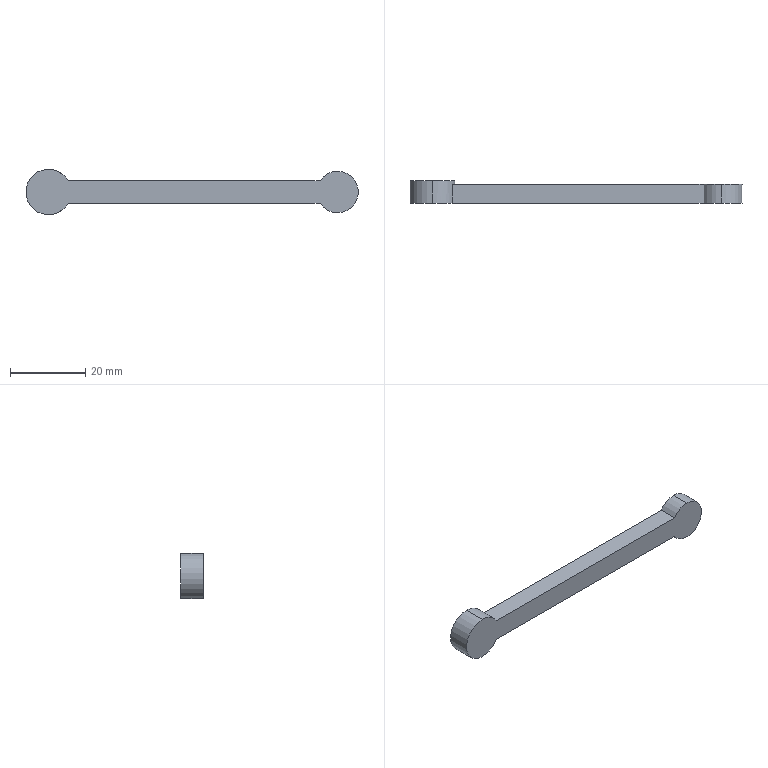Part | STEP file | 333_Default | 1 solid | 10 faces | box 88.1 x 6 x 12 mm | volume 3123 mm3 | cylinder 5 | plane 5 | commonest cylinder face diameters 11 x3 12 x2
STEP:
#1=CARTESIAN_POINT('',(0.,0.,0.));
#2=DIRECTION('',(0.,0.,1.));
#3=DIRECTION('',(1.,0.,0.));
#4=AXIS2_PLACEMENT_3D('',#1,#2,#3);
#5=CARTESIAN_POINT('',(38.3,0.,5.5));
#6=VERTEX_POINT('',#5);
#7=CARTESIAN_POINT('',(38.3,0.,-5.5));
#8=VERTEX_POINT('',#7);
#9=CARTESIAN_POINT('',(38.3,0.,0.));
#10=DIRECTION('',(0.,1.,0.));
#11=DIRECTION('',(0.,0.,1.));
#12=AXIS2_PLACEMENT_3D('',#9,#10,#11);
#13=CIRCLE('',#12,5.5);
#14=CARTESIAN_POINT('',(38.3,0.,0.));
#15=DIRECTION('',(0.,1.,0.));
#16=DIRECTION('',(0.,0.,1.));
#17=AXIS2_PLACEMENT_3D('',#14,#15,#16);
#18=CYLINDRICAL_SURFACE('',#17,5.5);
#19=CARTESIAN_POINT('',(0.,0.));
#20=DIRECTION('',(1.,0.));
#21=VECTOR('',#20,1.);
#22=LINE('',#19,#21);
#23=(GEOMETRIC_REPRESENTATION_CONTEXT(2)PARAMETRIC_REPRESENTATION_CONTEXT()REPRESENTATION_CONTEXT('',''));
#24=DEFINITIONAL_REPRESENTATION('',(#22),#23);
#25=PCURVE('',#18,#24);
#26=CARTESIAN_POINT('',(38.3,0.,0.));
#27=DIRECTION('',(0.,1.,0.));
#28=DIRECTION('',(0.,0.,1.));
#29=AXIS2_PLACEMENT_3D('',#26,#27,#28);
#30=PLANE('',#29);
#31=CARTESIAN_POINT('',(0.,0.));
#32=DIRECTION('',(1.,0.));
#33=AXIS2_PLACEMENT_2D('',#31,#32);
#34=CIRCLE('',#33,5.5);
#35=(GEOMETRIC_REPRESENTATION_CONTEXT(2)PARAMETRIC_REPRESENTATION_CONTEXT()REPRESENTATION_CONTEXT('',''));
#36=DEFINITIONAL_REPRESENTATION('',(#34),#35);
#37=PCURVE('',#30,#36);
#38=SURFACE_CURVE('',#13,(#25,#37),.PCURVE_S1.);
#39=EDGE_CURVE('',#6,#8,#38,.T.);
#40=ORIENTED_EDGE('',*,*,#39,.T.);
#41=CARTESIAN_POINT('',(38.3,5.,-5.5));
#42=VERTEX_POINT('',#41);
#43=CARTESIAN_POINT('',(38.3,0.,-5.5));
#44=DIRECTION('',(0.,1.,0.));
#45=VECTOR('',#44,1.);
#46=LINE('',#43,#45);
#47=CARTESIAN_POINT('',(3.142,0.));
#48=DIRECTION('',(0.,1.));
#49=VECTOR('',#48,1.);
#50=LINE('',#47,#49);
#51=(GEOMETRIC_REPRESENTATION_CONTEXT(2)PARAMETRIC_REPRESENTATION_CONTEXT()REPRESENTATION_CONTEXT('',''));
#52=DEFINITIONAL_REPRESENTATION('',(#50),#51);
#53=PCURVE('',#18,#52);
#54=CARTESIAN_POINT('',(38.3,0.,0.));
#55=DIRECTION('',(0.,1.,0.));
#56=DIRECTION('',(0.,0.,1.));
#57=AXIS2_PLACEMENT_3D('',#54,#55,#56);
#58=CYLINDRICAL_SURFACE('',#57,5.5);
#59=CARTESIAN_POINT('',(3.142,0.));
#60=DIRECTION('',(0.,1.));
#61=VECTOR('',#60,1.);
#62=LINE('',#59,#61);
#63=(GEOMETRIC_REPRESENTATION_CONTEXT(2)PARAMETRIC_REPRESENTATION_CONTEXT()REPRESENTATION_CONTEXT('',''));
#64=DEFINITIONAL_REPRESENTATION('',(#62),#63);
#65=PCURVE('',#58,#64);
#66=SURFACE_CURVE('',#46,(#53,#65),.PCURVE_S1.);
#67=EDGE_CURVE('',#8,#42,#66,.T.);
#68=ORIENTED_EDGE('',*,*,#67,.T.);
#69=CARTESIAN_POINT('',(38.3,5.,5.5));
#70=VERTEX_POINT('',#69);
#71=CARTESIAN_POINT('',(38.3,5.,0.));
#72=DIRECTION('',(0.,1.,0.));
#73=DIRECTION('',(0.,0.,1.));
#74=AXIS2_PLACEMENT_3D('',#71,#72,#73);
#75=CIRCLE('',#74,5.5);
#76=CARTESIAN_POINT('',(0.,5.));
#77=DIRECTION('',(1.,0.));
#78=VECTOR('',#77,1.);
#79=LINE('',#76,#78);
#80=(GEOMETRIC_REPRESENTATION_CONTEXT(2)PARAMETRIC_REPRESENTATION_CONTEXT()REPRESENTATION_CONTEXT('',''));
#81=DEFINITIONAL_REPRESENTATION('',(#79),#80);
#82=PCURVE('',#18,#81);
#83=CARTESIAN_POINT('',(38.3,5.,0.));
#84=DIRECTION('',(0.,1.,0.));
#85=DIRECTION('',(0.,0.,1.));
#86=AXIS2_PLACEMENT_3D('',#83,#84,#85);
#87=PLANE('',#86);
#88=CARTESIAN_POINT('',(0.,0.));
#89=DIRECTION('',(1.,0.));
#90=AXIS2_PLACEMENT_2D('',#88,#89);
#91=CIRCLE('',#90,5.5);
#92=(GEOMETRIC_REPRESENTATION_CONTEXT(2)PARAMETRIC_REPRESENTATION_CONTEXT()REPRESENTATION_CONTEXT('',''));
#93=DEFINITIONAL_REPRESENTATION('',(#91),#92);
#94=PCURVE('',#87,#93);
#95=SURFACE_CURVE('',#75,(#82,#94),.PCURVE_S1.);
#96=EDGE_CURVE('',#70,#42,#95,.T.);
#97=ORIENTED_EDGE('',*,*,#96,.F.);
#98=CARTESIAN_POINT('',(38.3,0.,5.5));
#99=DIRECTION('',(0.,1.,0.));
#100=VECTOR('',#99,1.);
#101=LINE('',#98,#100);
#102=CARTESIAN_POINT('',(0.,0.));
#103=DIRECTION('',(0.,1.));
#104=VECTOR('',#103,1.);
#105=LINE('',#102,#104);
#106=(GEOMETRIC_REPRESENTATION_CONTEXT(2)PARAMETRIC_REPRESENTATION_CONTEXT()REPRESENTATION_CONTEXT('',''));
#107=DEFINITIONAL_REPRESENTATION('',(#105),#106);
#108=PCURVE('',#18,#107);
#109=CARTESIAN_POINT('',(38.3,0.,0.));
#110=DIRECTION('',(0.,1.,0.));
#111=DIRECTION('',(0.,0.,1.));
#112=AXIS2_PLACEMENT_3D('',#109,#110,#111);
#113=CYLINDRICAL_SURFACE('',#112,5.5);
#114=CARTESIAN_POINT('',(6.283,0.));
#115=DIRECTION('',(0.,1.));
#116=VECTOR('',#115,1.);
#117=LINE('',#114,#116);
#118=(GEOMETRIC_REPRESENTATION_CONTEXT(2)PARAMETRIC_REPRESENTATION_CONTEXT()REPRESENTATION_CONTEXT('',''));
#119=DEFINITIONAL_REPRESENTATION('',(#117),#118);
#120=PCURVE('',#113,#119);
#121=SURFACE_CURVE('',#101,(#108,#120),.PCURVE_S1.);
#122=EDGE_CURVE('',#6,#70,#121,.T.);
#123=ORIENTED_EDGE('',*,*,#122,.F.);
#124=EDGE_LOOP('',(#40,#68,#97,#123));
#125=FACE_BOUND('',#124,.T.);
#126=ADVANCED_FACE('',(#125),#18,.T.);
#127=CARTESIAN_POINT('',(33.69,0.,3.));
#128=VERTEX_POINT('',#127);
#129=CARTESIAN_POINT('',(38.3,0.,0.));
#130=DIRECTION('',(0.,1.,0.));
#131=DIRECTION('',(0.,0.,1.));
#132=AXIS2_PLACEMENT_3D('',#129,#130,#131);
#133=CIRCLE('',#132,5.5);
#134=CARTESIAN_POINT('',(0.,0.));
#135=DIRECTION('',(1.,0.));
#136=VECTOR('',#135,1.);
#137=LINE('',#134,#136);
#138=(GEOMETRIC_REPRESENTATION_CONTEXT(2)PARAMETRIC_REPRESENTATION_CONTEXT()REPRESENTATION_CONTEXT('',''));
#139=DEFINITIONAL_REPRESENTATION('',(#137),#138);
#140=PCURVE('',#113,#139);
#141=CARTESIAN_POINT('',(0.,0.));
#142=DIRECTION('',(1.,0.));
#143=AXIS2_PLACEMENT_2D('',#141,#142);
#144=CIRCLE('',#143,5.5);
#145=(GEOMETRIC_REPRESENTATION_CONTEXT(2)PARAMETRIC_REPRESENTATION_CONTEXT()REPRESENTATION_CONTEXT('',''));
#146=DEFINITIONAL_REPRESENTATION('',(#144),#145);
#147=PCURVE('',#30,#146);
#148=SURFACE_CURVE('',#133,(#140,#147),.PCURVE_S1.);
#149=EDGE_CURVE('',#128,#6,#148,.T.);
#150=ORIENTED_EDGE('',*,*,#149,.T.);
#151=ORIENTED_EDGE('',*,*,#122,.T.);
#152=CARTESIAN_POINT('',(33.69,5.,3.));
#153=VERTEX_POINT('',#152);
#154=CARTESIAN_POINT('',(38.3,5.,0.));
#155=DIRECTION('',(0.,1.,0.));
#156=DIRECTION('',(0.,0.,1.));
#157=AXIS2_PLACEMENT_3D('',#154,#155,#156);
#158=CIRCLE('',#157,5.5);
#159=CARTESIAN_POINT('',(0.,5.));
#160=DIRECTION('',(1.,0.));
#161=VECTOR('',#160,1.);
#162=LINE('',#159,#161);
#163=(GEOMETRIC_REPRESENTATION_CONTEXT(2)PARAMETRIC_REPRESENTATION_CONTEXT()REPRESENTATION_CONTEXT('',''));
#164=DEFINITIONAL_REPRESENTATION('',(#162),#163);
#165=PCURVE('',#113,#164);
#166=CARTESIAN_POINT('',(0.,0.));
#167=DIRECTION('',(1.,0.));
#168=AXIS2_PLACEMENT_2D('',#166,#167);
#169=CIRCLE('',#168,5.5);
#170=(GEOMETRIC_REPRESENTATION_CONTEXT(2)PARAMETRIC_REPRESENTATION_CONTEXT()REPRESENTATION_CONTEXT('',''));
#171=DEFINITIONAL_REPRESENTATION('',(#169),#170);
#172=PCURVE('',#87,#171);
#173=SURFACE_CURVE('',#158,(#165,#172),.PCURVE_S1.);
#174=EDGE_CURVE('',#153,#70,#173,.T.);
#175=ORIENTED_EDGE('',*,*,#174,.F.);
#176=CARTESIAN_POINT('',(33.69,0.,3.));
#177=DIRECTION('',(0.,1.,0.));
#178=VECTOR('',#177,1.);
#179=LINE('',#176,#178);
#180=CARTESIAN_POINT('',(5.289,0.));
#181=DIRECTION('',(0.,1.));
#182=VECTOR('',#181,1.);
#183=LINE('',#180,#182);
#184=(GEOMETRIC_REPRESENTATION_CONTEXT(2)PARAMETRIC_REPRESENTATION_CONTEXT()REPRESENTATION_CONTEXT('',''));
#185=DEFINITIONAL_REPRESENTATION('',(#183),#184);
#186=PCURVE('',#113,#185);
#187=CARTESIAN_POINT('',(-33.104,0.,3.));
#188=DIRECTION('',(0.,0.,1.));
#189=DIRECTION('',(1.,0.,0.));
#190=AXIS2_PLACEMENT_3D('',#187,#188,#189);
#191=PLANE('',#190);
#192=CARTESIAN_POINT('',(66.794,0.));
#193=DIRECTION('',(0.,1.));
#194=VECTOR('',#193,1.);
#195=LINE('',#192,#194);
#196=(GEOMETRIC_REPRESENTATION_CONTEXT(2)PARAMETRIC_REPRESENTATION_CONTEXT()REPRESENTATION_CONTEXT('',''));
#197=DEFINITIONAL_REPRESENTATION('',(#195),#196);
#198=PCURVE('',#191,#197);
#199=SURFACE_CURVE('',#179,(#186,#198),.PCURVE_S1.);
#200=EDGE_CURVE('',#128,#153,#199,.T.);
#201=ORIENTED_EDGE('',*,*,#200,.F.);
#202=EDGE_LOOP('',(#150,#151,#175,#201));
#203=FACE_BOUND('',#202,.T.);
#204=ADVANCED_FACE('',(#203),#113,.T.);
#205=CARTESIAN_POINT('',(-38.3,6.,6.));
#206=VERTEX_POINT('',#205);
#207=CARTESIAN_POINT('',(-38.3,6.,-6.));
#208=VERTEX_POINT('',#207);
#209=CARTESIAN_POINT('',(-38.3,6.,0.));
#210=DIRECTION('',(0.,1.,0.));
#211=DIRECTION('',(0.,0.,1.));
#212=AXIS2_PLACEMENT_3D('',#209,#210,#211);
#213=CIRCLE('',#212,6.);
#214=CARTESIAN_POINT('',(-38.3,5.,0.));
#215=DIRECTION('',(0.,-1.,0.));
#216=DIRECTION('',(0.,0.,-1.));
#217=AXIS2_PLACEMENT_3D('',#214,#215,#216);
#218=CYLINDRICAL_SURFACE('',#217,6.);
#219=CARTESIAN_POINT('',(3.142,-1.));
#220=DIRECTION('',(-1.,0.));
#221=VECTOR('',#220,1.);
#222=LINE('',#219,#221);
#223=(GEOMETRIC_REPRESENTATION_CONTEXT(2)PARAMETRIC_REPRESENTATION_CONTEXT()REPRESENTATION_CONTEXT('',''));
#224=DEFINITIONAL_REPRESENTATION('',(#222),#223);
#225=PCURVE('',#218,#224);
#226=CARTESIAN_POINT('',(-38.3,6.,0.));
#227=DIRECTION('',(0.,1.,0.));
#228=DIRECTION('',(0.,0.,1.));
#229=AXIS2_PLACEMENT_3D('',#226,#227,#228);
#230=PLANE('',#229);
#231=CARTESIAN_POINT('',(0.,0.));
#232=DIRECTION('',(1.,0.));
#233=AXIS2_PLACEMENT_2D('',#231,#232);
#234=CIRCLE('',#233,6.);
#235=(GEOMETRIC_REPRESENTATION_CONTEXT(2)PARAMETRIC_REPRESENTATION_CONTEXT()REPRESENTATION_CONTEXT('',''));
#236=DEFINITIONAL_REPRESENTATION('',(#234),#235);
#237=PCURVE('',#230,#236);
#238=SURFACE_CURVE('',#213,(#225,#237),.PCURVE_S1.);
#239=EDGE_CURVE('',#206,#208,#238,.T.);
#240=ORIENTED_EDGE('',*,*,#239,.F.);
#241=CARTESIAN_POINT('',(-38.3,0.,6.));
#242=VERTEX_POINT('',#241);
#243=CARTESIAN_POINT('',(-38.3,5.,6.));
#244=DIRECTION('',(0.,-1.,0.));
#245=VECTOR('',#244,1.);
#246=LINE('',#243,#245);
#247=CARTESIAN_POINT('',(3.142,0.));
#248=DIRECTION('',(0.,1.));
#249=VECTOR('',#248,1.);
#250=LINE('',#247,#249);
#251=(GEOMETRIC_REPRESENTATION_CONTEXT(2)PARAMETRIC_REPRESENTATION_CONTEXT()REPRESENTATION_CONTEXT('',''));
#252=DEFINITIONAL_REPRESENTATION('',(#250),#251);
#253=PCURVE('',#218,#252);
#254=CARTESIAN_POINT('',(-38.3,5.,0.));
#255=DIRECTION('',(0.,-1.,0.));
#256=DIRECTION('',(0.,0.,-1.));
#257=AXIS2_PLACEMENT_3D('',#254,#255,#256);
#258=CYLINDRICAL_SURFACE('',#257,6.);
#259=CARTESIAN_POINT('',(3.142,0.));
#260=DIRECTION('',(0.,1.));
#261=VECTOR('',#260,1.);
#262=LINE('',#259,#261);
#263=(GEOMETRIC_REPRESENTATION_CONTEXT(2)PARAMETRIC_REPRESENTATION_CONTEXT()REPRESENTATION_CONTEXT('',''));
#264=DEFINITIONAL_REPRESENTATION('',(#262),#263);
#265=PCURVE('',#258,#264);
#266=SURFACE_CURVE('',#246,(#253,#265),.PCURVE_S1.);
#267=EDGE_CURVE('',#206,#242,#266,.T.);
#268=ORIENTED_EDGE('',*,*,#267,.T.);
#269=CARTESIAN_POINT('',(-33.104,0.,3.));
#270=VERTEX_POINT('',#269);
#271=CARTESIAN_POINT('',(-38.3,0.,0.));
#272=DIRECTION('',(0.,1.,0.));
#273=DIRECTION('',(0.,0.,1.));
#274=AXIS2_PLACEMENT_3D('',#271,#272,#273);
#275=CIRCLE('',#274,6.);
#276=CARTESIAN_POINT('',(3.142,5.));
#277=DIRECTION('',(-1.,0.));
#278=VECTOR('',#277,1.);
#279=LINE('',#276,#278);
#280=(GEOMETRIC_REPRESENTATION_CONTEXT(2)PARAMETRIC_REPRESENTATION_CONTEXT()REPRESENTATION_CONTEXT('',''));
#281=DEFINITIONAL_REPRESENTATION('',(#279),#280);
#282=PCURVE('',#218,#281);
#283=CARTESIAN_POINT('',(0.,-76.6));
#284=DIRECTION('',(1.,0.));
#285=AXIS2_PLACEMENT_2D('',#283,#284);
#286=CIRCLE('',#285,6.);
#287=(GEOMETRIC_REPRESENTATION_CONTEXT(2)PARAMETRIC_REPRESENTATION_CONTEXT()REPRESENTATION_CONTEXT('',''));
#288=DEFINITIONAL_REPRESENTATION('',(#286),#287);
#289=PCURVE('',#30,#288);
#290=SURFACE_CURVE('',#275,(#282,#289),.PCURVE_S1.);
#291=EDGE_CURVE('',#242,#270,#290,.T.);
#292=ORIENTED_EDGE('',*,*,#291,.T.);
#293=CARTESIAN_POINT('',(-33.104,5.,3.));
#294=VERTEX_POINT('',#293);
#295=CARTESIAN_POINT('',(-33.104,0.,3.));
#296=DIRECTION('',(0.,1.,0.));
#297=VECTOR('',#296,1.);
#298=LINE('',#295,#297);
#299=CARTESIAN_POINT('',(2.094,5.));
#300=DIRECTION('',(0.,-1.));
#301=VECTOR('',#300,1.);
#302=LINE('',#299,#301);
#303=(GEOMETRIC_REPRESENTATION_CONTEXT(2)PARAMETRIC_REPRESENTATION_CONTEXT()REPRESENTATION_CONTEXT('',''));
#304=DEFINITIONAL_REPRESENTATION('',(#302),#303);
#305=PCURVE('',#218,#304);
#306=CARTESIAN_POINT('',(0.,0.));
#307=DIRECTION('',(0.,1.));
#308=VECTOR('',#307,1.);
#309=LINE('',#306,#308);
#310=(GEOMETRIC_REPRESENTATION_CONTEXT(2)PARAMETRIC_REPRESENTATION_CONTEXT()REPRESENTATION_CONTEXT('',''));
#311=DEFINITIONAL_REPRESENTATION('',(#309),#310);
#312=PCURVE('',#191,#311);
#313=SURFACE_CURVE('',#298,(#305,#312),.PCURVE_S1.);
#314=EDGE_CURVE('',#270,#294,#313,.T.);
#315=ORIENTED_EDGE('',*,*,#314,.T.);
#316=CARTESIAN_POINT('',(-33.104,5.,-3.));
#317=VERTEX_POINT('',#316);
#318=CARTESIAN_POINT('',(-38.3,5.,0.));
#319=DIRECTION('',(0.,1.,0.));
#320=DIRECTION('',(0.,0.,1.));
#321=AXIS2_PLACEMENT_3D('',#318,#319,#320);
#322=CIRCLE('',#321,6.);
#323=CARTESIAN_POINT('',(3.142,0.));
#324=DIRECTION('',(-1.,0.));
#325=VECTOR('',#324,1.);
#326=LINE('',#323,#325);
#327=(GEOMETRIC_REPRESENTATION_CONTEXT(2)PARAMETRIC_REPRESENTATION_CONTEXT()REPRESENTATION_CONTEXT('',''));
#328=DEFINITIONAL_REPRESENTATION('',(#326),#327);
#329=PCURVE('',#218,#328);
#330=CARTESIAN_POINT('',(0.,-76.6));
#331=DIRECTION('',(1.,0.));
#332=AXIS2_PLACEMENT_2D('',#330,#331);
#333=CIRCLE('',#332,6.);
#334=(GEOMETRIC_REPRESENTATION_CONTEXT(2)PARAMETRIC_REPRESENTATION_CONTEXT()REPRESENTATION_CONTEXT('',''));
#335=DEFINITIONAL_REPRESENTATION('',(#333),#334);
#336=PCURVE('',#87,#335);
#337=SURFACE_CURVE('',#322,(#329,#336),.PCURVE_S1.);
#338=EDGE_CURVE('',#294,#317,#337,.T.);
#339=ORIENTED_EDGE('',*,*,#338,.T.);
#340=CARTESIAN_POINT('',(-33.104,0.,-3.));
#341=VERTEX_POINT('',#340);
#342=CARTESIAN_POINT('',(-33.104,0.,-3.));
#343=DIRECTION('',(0.,1.,0.));
#344=VECTOR('',#343,1.);
#345=LINE('',#342,#344);
#346=CARTESIAN_POINT('',(1.047,5.));
#347=DIRECTION('',(0.,-1.));
#348=VECTOR('',#347,1.);
#349=LINE('',#346,#348);
#350=(GEOMETRIC_REPRESENTATION_CONTEXT(2)PARAMETRIC_REPRESENTATION_CONTEXT()REPRESENTATION_CONTEXT('',''));
#351=DEFINITIONAL_REPRESENTATION('',(#349),#350);
#352=PCURVE('',#218,#351);
#353=CARTESIAN_POINT('',(-33.104,0.,-3.));
#354=DIRECTION('',(0.,0.,-1.));
#355=DIRECTION('',(-1.,0.,0.));
#356=AXIS2_PLACEMENT_3D('',#353,#354,#355);
#357=PLANE('',#356);
#358=CARTESIAN_POINT('',(0.,0.));
#359=DIRECTION('',(0.,1.));
#360=VECTOR('',#359,1.);
#361=LINE('',#358,#360);
#362=(GEOMETRIC_REPRESENTATION_CONTEXT(2)PARAMETRIC_REPRESENTATION_CONTEXT()REPRESENTATION_CONTEXT('',''));
#363=DEFINITIONAL_REPRESENTATION('',(#361),#362);
#364=PCURVE('',#357,#363);
#365=SURFACE_CURVE('',#345,(#352,#364),.PCURVE_S1.);
#366=EDGE_CURVE('',#341,#317,#365,.T.);
#367=ORIENTED_EDGE('',*,*,#366,.F.);
#368=CARTESIAN_POINT('',(-38.3,0.,-6.));
#369=VERTEX_POINT('',#368);
#370=CARTESIAN_POINT('',(-38.3,0.,0.));
#371=DIRECTION('',(0.,1.,0.));
#372=DIRECTION('',(0.,0.,1.));
#373=AXIS2_PLACEMENT_3D('',#370,#371,#372);
#374=CIRCLE('',#373,6.);
#375=CARTESIAN_POINT('',(3.142,5.));
#376=DIRECTION('',(-1.,0.));
#377=VECTOR('',#376,1.);
#378=LINE('',#375,#377);
#379=(GEOMETRIC_REPRESENTATION_CONTEXT(2)PARAMETRIC_REPRESENTATION_CONTEXT()REPRESENTATION_CONTEXT('',''));
#380=DEFINITIONAL_REPRESENTATION('',(#378),#379);
#381=PCURVE('',#218,#380);
#382=CARTESIAN_POINT('',(0.,-76.6));
#383=DIRECTION('',(1.,0.));
#384=AXIS2_PLACEMENT_2D('',#382,#383);
#385=CIRCLE('',#384,6.);
#386=(GEOMETRIC_REPRESENTATION_CONTEXT(2)PARAMETRIC_REPRESENTATION_CONTEXT()REPRESENTATION_CONTEXT('',''));
#387=DEFINITIONAL_REPRESENTATION('',(#385),#386);
#388=PCURVE('',#30,#387);
#389=SURFACE_CURVE('',#374,(#381,#388),.PCURVE_S1.);
#390=EDGE_CURVE('',#341,#369,#389,.T.);
#391=ORIENTED_EDGE('',*,*,#390,.T.);
#392=CARTESIAN_POINT('',(-38.3,5.,-6.));
#393=DIRECTION('',(0.,-1.,0.));
#394=VECTOR('',#393,1.);
#395=LINE('',#392,#394);
#396=CARTESIAN_POINT('',(0.,0.));
#397=DIRECTION('',(0.,1.));
#398=VECTOR('',#397,1.);
#399=LINE('',#396,#398);
#400=(GEOMETRIC_REPRESENTATION_CONTEXT(2)PARAMETRIC_REPRESENTATION_CONTEXT()REPRESENTATION_CONTEXT('',''));
#401=DEFINITIONAL_REPRESENTATION('',(#399),#400);
#402=PCURVE('',#218,#401);
#403=CARTESIAN_POINT('',(6.283,0.));
#404=DIRECTION('',(0.,1.));
#405=VECTOR('',#404,1.);
#406=LINE('',#403,#405);
#407=(GEOMETRIC_REPRESENTATION_CONTEXT(2)PARAMETRIC_REPRESENTATION_CONTEXT()REPRESENTATION_CONTEXT('',''));
#408=DEFINITIONAL_REPRESENTATION('',(#406),#407);
#409=PCURVE('',#258,#408);
#410=SURFACE_CURVE('',#395,(#402,#409),.PCURVE_S1.);
#411=EDGE_CURVE('',#208,#369,#410,.T.);
#412=ORIENTED_EDGE('',*,*,#411,.F.);
#413=EDGE_LOOP('',(#240,#268,#292,#315,#339,#367,#391,#412));
#414=FACE_BOUND('',#413,.T.);
#415=ADVANCED_FACE('',(#414),#218,.T.);
#416=ORIENTED_EDGE('',*,*,#338,.F.);
#417=CARTESIAN_POINT('',(-33.104,5.,3.));
#418=DIRECTION('',(1.,0.,0.));
#419=VECTOR('',#418,1.);
#420=LINE('',#417,#419);
#421=CARTESIAN_POINT('',(3.,-71.404));
#422=DIRECTION('',(0.,1.));
#423=VECTOR('',#422,1.);
#424=LINE('',#421,#423);
#425=(GEOMETRIC_REPRESENTATION_CONTEXT(2)PARAMETRIC_REPRESENTATION_CONTEXT()REPRESENTATION_CONTEXT('',''));
#426=DEFINITIONAL_REPRESENTATION('',(#424),#425);
#427=PCURVE('',#87,#426);
#428=CARTESIAN_POINT('',(0.,5.));
#429=DIRECTION('',(1.,0.));
#430=VECTOR('',#429,1.);
#431=LINE('',#428,#430);
#432=(GEOMETRIC_REPRESENTATION_CONTEXT(2)PARAMETRIC_REPRESENTATION_CONTEXT()REPRESENTATION_CONTEXT('',''));
#433=DEFINITIONAL_REPRESENTATION('',(#431),#432);
#434=PCURVE('',#191,#433);
#435=SURFACE_CURVE('',#420,(#427,#434),.PCURVE_S1.);
#436=EDGE_CURVE('',#294,#153,#435,.T.);
#437=ORIENTED_EDGE('',*,*,#436,.T.);
#438=ORIENTED_EDGE('',*,*,#174,.T.);
#439=ORIENTED_EDGE('',*,*,#96,.T.);
#440=CARTESIAN_POINT('',(33.69,5.,-3.));
#441=VERTEX_POINT('',#440);
#442=CARTESIAN_POINT('',(38.3,5.,0.));
#443=DIRECTION('',(0.,1.,0.));
#444=DIRECTION('',(0.,0.,1.));
#445=AXIS2_PLACEMENT_3D('',#442,#443,#444);
#446=CIRCLE('',#445,5.5);
#447=CARTESIAN_POINT('',(0.,0.));
#448=DIRECTION('',(1.,0.));
#449=AXIS2_PLACEMENT_2D('',#447,#448);
#450=CIRCLE('',#449,5.5);
#451=(GEOMETRIC_REPRESENTATION_CONTEXT(2)PARAMETRIC_REPRESENTATION_CONTEXT()REPRESENTATION_CONTEXT('',''));
#452=DEFINITIONAL_REPRESENTATION('',(#450),#451);
#453=PCURVE('',#87,#452);
#454=CARTESIAN_POINT('',(0.,5.));
#455=DIRECTION('',(1.,0.));
#456=VECTOR('',#455,1.);
#457=LINE('',#454,#456);
#458=(GEOMETRIC_REPRESENTATION_CONTEXT(2)PARAMETRIC_REPRESENTATION_CONTEXT()REPRESENTATION_CONTEXT('',''));
#459=DEFINITIONAL_REPRESENTATION('',(#457),#458);
#460=PCURVE('',#58,#459);
#461=SURFACE_CURVE('',#446,(#453,#460),.PCURVE_S1.);
#462=EDGE_CURVE('',#42,#441,#461,.T.);
#463=ORIENTED_EDGE('',*,*,#462,.T.);
#464=CARTESIAN_POINT('',(-33.104,5.,-3.));
#465=DIRECTION('',(-1.,0.,0.));
#466=VECTOR('',#465,1.);
#467=LINE('',#464,#466);
#468=CARTESIAN_POINT('',(-3.,-71.404));
#469=DIRECTION('',(0.,-1.));
#470=VECTOR('',#469,1.);
#471=LINE('',#468,#470);
#472=(GEOMETRIC_REPRESENTATION_CONTEXT(2)PARAMETRIC_REPRESENTATION_CONTEXT()REPRESENTATION_CONTEXT('',''));
#473=DEFINITIONAL_REPRESENTATION('',(#471),#472);
#474=PCURVE('',#87,#473);
#475=CARTESIAN_POINT('',(0.,5.));
#476=DIRECTION('',(1.,0.));
#477=VECTOR('',#476,1.);
#478=LINE('',#475,#477);
#479=(GEOMETRIC_REPRESENTATION_CONTEXT(2)PARAMETRIC_REPRESENTATION_CONTEXT()REPRESENTATION_CONTEXT('',''));
#480=DEFINITIONAL_REPRESENTATION('',(#478),#479);
#481=PCURVE('',#357,#480);
#482=SURFACE_CURVE('',#467,(#474,#481),.PCURVE_S1.);
#483=EDGE_CURVE('',#441,#317,#482,.T.);
#484=ORIENTED_EDGE('',*,*,#483,.T.);
#485=EDGE_LOOP('',(#416,#437,#438,#439,#463,#484));
#486=FACE_BOUND('',#485,.T.);
#487=ADVANCED_FACE('',(#486),#87,.T.);
#488=CARTESIAN_POINT('',(-33.104,0.,3.));
#489=DIRECTION('',(1.,0.,0.));
#490=VECTOR('',#489,1.);
#491=LINE('',#488,#490);
#492=CARTESIAN_POINT('',(3.,-71.404));
#493=DIRECTION('',(0.,1.));
#494=VECTOR('',#493,1.);
#495=LINE('',#492,#494);
#496=(GEOMETRIC_REPRESENTATION_CONTEXT(2)PARAMETRIC_REPRESENTATION_CONTEXT()REPRESENTATION_CONTEXT('',''));
#497=DEFINITIONAL_REPRESENTATION('',(#495),#496);
#498=PCURVE('',#30,#497);
#499=CARTESIAN_POINT('',(0.,0.));
#500=DIRECTION('',(1.,0.));
#501=VECTOR('',#500,1.);
#502=LINE('',#499,#501);
#503=(GEOMETRIC_REPRESENTATION_CONTEXT(2)PARAMETRIC_REPRESENTATION_CONTEXT()REPRESENTATION_CONTEXT('',''));
#504=DEFINITIONAL_REPRESENTATION('',(#502),#503);
#505=PCURVE('',#191,#504);
#506=SURFACE_CURVE('',#491,(#498,#505),.PCURVE_S1.);
#507=EDGE_CURVE('',#270,#128,#506,.T.);
#508=ORIENTED_EDGE('',*,*,#507,.F.);
#509=ORIENTED_EDGE('',*,*,#291,.F.);
#510=CARTESIAN_POINT('',(-38.3,0.,0.));
#511=DIRECTION('',(0.,1.,0.));
#512=DIRECTION('',(0.,0.,1.));
#513=AXIS2_PLACEMENT_3D('',#510,#511,#512);
#514=CIRCLE('',#513,6.);
#515=CARTESIAN_POINT('',(0.,-76.6));
#516=DIRECTION('',(1.,0.));
#517=AXIS2_PLACEMENT_2D('',#515,#516);
#518=CIRCLE('',#517,6.);
#519=(GEOMETRIC_REPRESENTATION_CONTEXT(2)PARAMETRIC_REPRESENTATION_CONTEXT()REPRESENTATION_CONTEXT('',''));
#520=DEFINITIONAL_REPRESENTATION('',(#518),#519);
#521=PCURVE('',#30,#520);
#522=CARTESIAN_POINT('',(9.425,5.));
#523=DIRECTION('',(-1.,0.));
#524=VECTOR('',#523,1.);
#525=LINE('',#522,#524);
#526=(GEOMETRIC_REPRESENTATION_CONTEXT(2)PARAMETRIC_REPRESENTATION_CONTEXT()REPRESENTATION_CONTEXT('',''));
#527=DEFINITIONAL_REPRESENTATION('',(#525),#526);
#528=PCURVE('',#258,#527);
#529=SURFACE_CURVE('',#514,(#521,#528),.PCURVE_S1.);
#530=EDGE_CURVE('',#369,#242,#529,.T.);
#531=ORIENTED_EDGE('',*,*,#530,.F.);
#532=ORIENTED_EDGE('',*,*,#390,.F.);
#533=CARTESIAN_POINT('',(33.69,0.,-3.));
#534=VERTEX_POINT('',#533);
#535=CARTESIAN_POINT('',(-33.104,0.,-3.));
#536=DIRECTION('',(-1.,0.,0.));
#537=VECTOR('',#536,1.);
#538=LINE('',#535,#537);
#539=CARTESIAN_POINT('',(-3.,-71.404));
#540=DIRECTION('',(0.,-1.));
#541=VECTOR('',#540,1.);
#542=LINE('',#539,#541);
#543=(GEOMETRIC_REPRESENTATION_CONTEXT(2)PARAMETRIC_REPRESENTATION_CONTEXT()REPRESENTATION_CONTEXT('',''));
#544=DEFINITIONAL_REPRESENTATION('',(#542),#543);
#545=PCURVE('',#30,#544);
#546=CARTESIAN_POINT('',(0.,0.));
#547=DIRECTION('',(1.,0.));
#548=VECTOR('',#547,1.);
#549=LINE('',#546,#548);
#550=(GEOMETRIC_REPRESENTATION_CONTEXT(2)PARAMETRIC_REPRESENTATION_CONTEXT()REPRESENTATION_CONTEXT('',''));
#551=DEFINITIONAL_REPRESENTATION('',(#549),#550);
#552=PCURVE('',#357,#551);
#553=SURFACE_CURVE('',#538,(#545,#552),.PCURVE_S1.);
#554=EDGE_CURVE('',#534,#341,#553,.T.);
#555=ORIENTED_EDGE('',*,*,#554,.F.);
#556=CARTESIAN_POINT('',(38.3,0.,0.));
#557=DIRECTION('',(0.,1.,0.));
#558=DIRECTION('',(0.,0.,1.));
#559=AXIS2_PLACEMENT_3D('',#556,#557,#558);
#560=CIRCLE('',#559,5.5);
#561=CARTESIAN_POINT('',(0.,0.));
#562=DIRECTION('',(1.,0.));
#563=AXIS2_PLACEMENT_2D('',#561,#562);
#564=CIRCLE('',#563,5.5);
#565=(GEOMETRIC_REPRESENTATION_CONTEXT(2)PARAMETRIC_REPRESENTATION_CONTEXT()REPRESENTATION_CONTEXT('',''));
#566=DEFINITIONAL_REPRESENTATION('',(#564),#565);
#567=PCURVE('',#30,#566);
#568=CARTESIAN_POINT('',(0.,0.));
#569=DIRECTION('',(1.,0.));
#570=VECTOR('',#569,1.);
#571=LINE('',#568,#570);
#572=(GEOMETRIC_REPRESENTATION_CONTEXT(2)PARAMETRIC_REPRESENTATION_CONTEXT()REPRESENTATION_CONTEXT('',''));
#573=DEFINITIONAL_REPRESENTATION('',(#571),#572);
#574=PCURVE('',#58,#573);
#575=SURFACE_CURVE('',#560,(#567,#574),.PCURVE_S1.);
#576=EDGE_CURVE('',#8,#534,#575,.T.);
#577=ORIENTED_EDGE('',*,*,#576,.F.);
#578=ORIENTED_EDGE('',*,*,#39,.F.);
#579=ORIENTED_EDGE('',*,*,#149,.F.);
#580=EDGE_LOOP('',(#508,#509,#531,#532,#555,#577,#578,#579));
#581=FACE_BOUND('',#580,.T.);
#582=ADVANCED_FACE('',(#581),#30,.F.);
#583=ORIENTED_EDGE('',*,*,#267,.F.);
#584=CARTESIAN_POINT('',(-38.3,6.,0.));
#585=DIRECTION('',(0.,1.,0.));
#586=DIRECTION('',(0.,0.,1.));
#587=AXIS2_PLACEMENT_3D('',#584,#585,#586);
#588=CIRCLE('',#587,6.);
#589=CARTESIAN_POINT('',(9.425,-1.));
#590=DIRECTION('',(-1.,0.));
#591=VECTOR('',#590,1.);
#592=LINE('',#589,#591);
#593=(GEOMETRIC_REPRESENTATION_CONTEXT(2)PARAMETRIC_REPRESENTATION_CONTEXT()REPRESENTATION_CONTEXT('',''));
#594=DEFINITIONAL_REPRESENTATION('',(#592),#593);
#595=PCURVE('',#258,#594);
#596=CARTESIAN_POINT('',(0.,0.));
#597=DIRECTION('',(1.,0.));
#598=AXIS2_PLACEMENT_2D('',#596,#597);
#599=CIRCLE('',#598,6.);
#600=(GEOMETRIC_REPRESENTATION_CONTEXT(2)PARAMETRIC_REPRESENTATION_CONTEXT()REPRESENTATION_CONTEXT('',''));
#601=DEFINITIONAL_REPRESENTATION('',(#599),#600);
#602=PCURVE('',#230,#601);
#603=SURFACE_CURVE('',#588,(#595,#602),.PCURVE_S1.);
#604=EDGE_CURVE('',#208,#206,#603,.T.);
#605=ORIENTED_EDGE('',*,*,#604,.F.);
#606=ORIENTED_EDGE('',*,*,#411,.T.);
#607=ORIENTED_EDGE('',*,*,#530,.T.);
#608=EDGE_LOOP('',(#583,#605,#606,#607));
#609=FACE_BOUND('',#608,.T.);
#610=ADVANCED_FACE('',(#609),#258,.T.);
#611=ORIENTED_EDGE('',*,*,#67,.F.);
#612=ORIENTED_EDGE('',*,*,#576,.T.);
#613=CARTESIAN_POINT('',(33.69,0.,-3.));
#614=DIRECTION('',(0.,1.,0.));
#615=VECTOR('',#614,1.);
#616=LINE('',#613,#615);
#617=CARTESIAN_POINT('',(4.135,0.));
#618=DIRECTION('',(0.,1.));
#619=VECTOR('',#618,1.);
#620=LINE('',#617,#619);
#621=(GEOMETRIC_REPRESENTATION_CONTEXT(2)PARAMETRIC_REPRESENTATION_CONTEXT()REPRESENTATION_CONTEXT('',''));
#622=DEFINITIONAL_REPRESENTATION('',(#620),#621);
#623=PCURVE('',#58,#622);
#624=CARTESIAN_POINT('',(-66.794,0.));
#625=DIRECTION('',(0.,1.));
#626=VECTOR('',#625,1.);
#627=LINE('',#624,#626);
#628=(GEOMETRIC_REPRESENTATION_CONTEXT(2)PARAMETRIC_REPRESENTATION_CONTEXT()REPRESENTATION_CONTEXT('',''));
#629=DEFINITIONAL_REPRESENTATION('',(#627),#628);
#630=PCURVE('',#357,#629);
#631=SURFACE_CURVE('',#616,(#623,#630),.PCURVE_S1.);
#632=EDGE_CURVE('',#534,#441,#631,.T.);
#633=ORIENTED_EDGE('',*,*,#632,.T.);
#634=ORIENTED_EDGE('',*,*,#462,.F.);
#635=EDGE_LOOP('',(#611,#612,#633,#634));
#636=FACE_BOUND('',#635,.T.);
#637=ADVANCED_FACE('',(#636),#58,.T.);
#638=ORIENTED_EDGE('',*,*,#436,.F.);
#639=ORIENTED_EDGE('',*,*,#314,.F.);
#640=ORIENTED_EDGE('',*,*,#507,.T.);
#641=ORIENTED_EDGE('',*,*,#200,.T.);
#642=EDGE_LOOP('',(#638,#639,#640,#641));
#643=FACE_BOUND('',#642,.T.);
#644=ADVANCED_FACE('',(#643),#191,.T.);
#645=ORIENTED_EDGE('',*,*,#483,.F.);
#646=ORIENTED_EDGE('',*,*,#632,.F.);
#647=ORIENTED_EDGE('',*,*,#554,.T.);
#648=ORIENTED_EDGE('',*,*,#366,.T.);
#649=EDGE_LOOP('',(#645,#646,#647,#648));
#650=FACE_BOUND('',#649,.T.);
#651=ADVANCED_FACE('',(#650),#357,.T.);
#652=ORIENTED_EDGE('',*,*,#604,.T.);
#653=ORIENTED_EDGE('',*,*,#239,.T.);
#654=EDGE_LOOP('',(#652,#653));
#655=FACE_BOUND('',#654,.T.);
#656=ADVANCED_FACE('',(#655),#230,.T.);
#657=CLOSED_SHELL('',(#126,#204,#415,#487,#582,#610,#637,#644,#651,#656));
#658=MANIFOLD_SOLID_BREP('',#657);
#659=(LENGTH_UNIT()NAMED_UNIT(*)SI_UNIT(.MILLI.,.METRE.));
#660=UNCERTAINTY_MEASURE_WITH_UNIT(LENGTH_MEASURE(0.0000001),#659,'','');
#661=(NAMED_UNIT(*)PLANE_ANGLE_UNIT()SI_UNIT($,.RADIAN.));
#662=(NAMED_UNIT(*)SI_UNIT($,.STERADIAN.)SOLID_ANGLE_UNIT());
#663=(GEOMETRIC_REPRESENTATION_CONTEXT(3)GLOBAL_UNCERTAINTY_ASSIGNED_CONTEXT((#660))GLOBAL_UNIT_ASSIGNED_CONTEXT((#659,#661,#662))REPRESENTATION_CONTEXT('',''));
#664=ADVANCED_BREP_SHAPE_REPRESENTATION('',(#4,#658),#663);